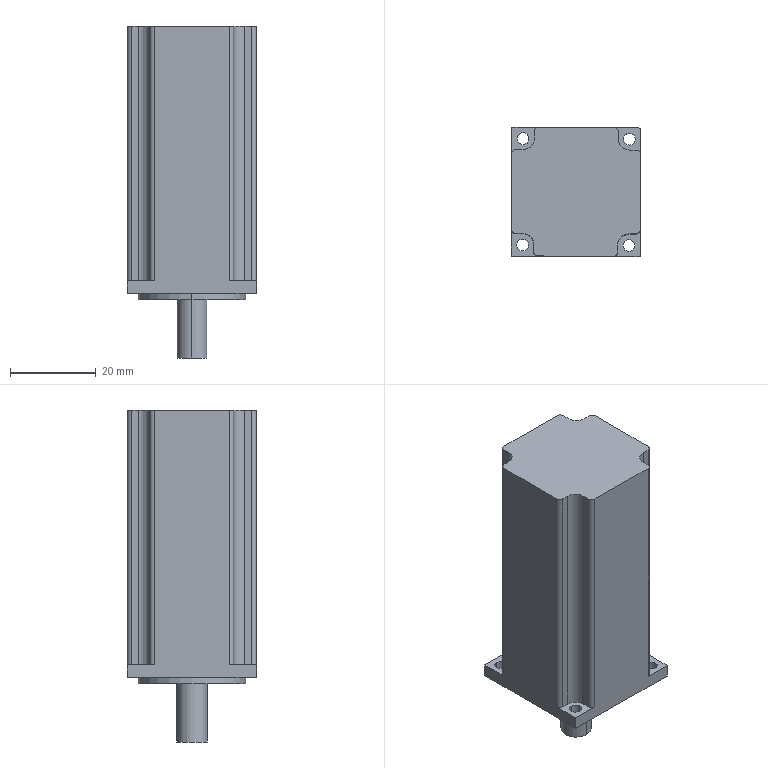Part | STEP file | 2026.6.15-Main Assembly图.sldasm-Part-155 | 1 solid | 47 faces | box 30.153 x 30.153 x 77.25 mm | volume 50923 mm3 | cylinder 27 | plane 20 | commonest cylinder face diameters 2 x10 2.75 x8 5.251 x5 7 x2 25 x2